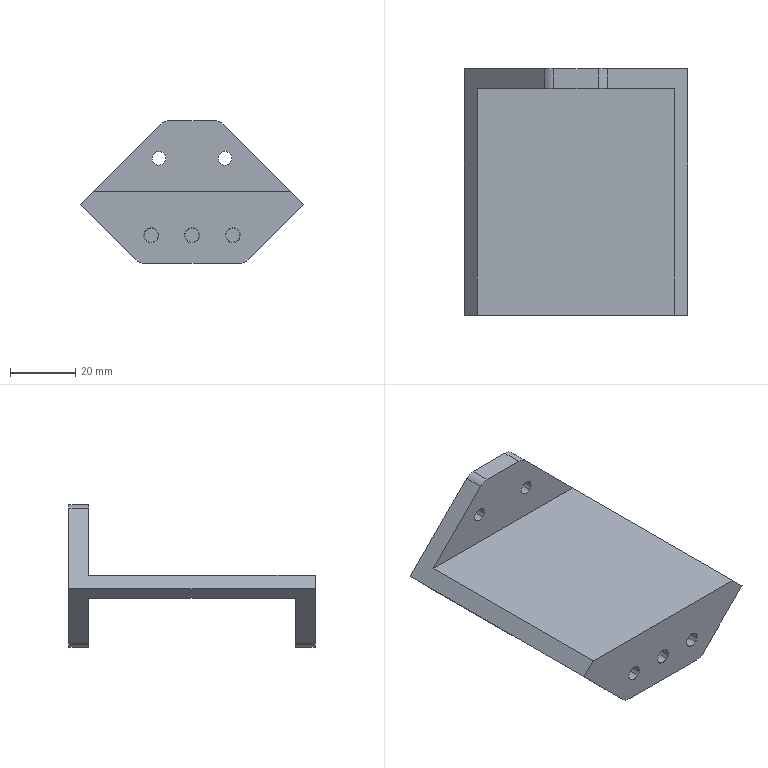NC program | NX | posted with a generic post | part box 68.307 x 75.3 x 43.668 mm
Lines 1 to 80 of 6865:
N10 G17 G21 G94 G90
(FLOOR_WALL_COPY_COPY , TOOL : D80)
N12 T19 M6
N14 G54
N16 G17 G0 G90 X-79.153 Y37.647 B0. C0. S6500 M3
N18 G43 Z30. H19
N20 Z9.
N22 G94 G1 Z6. F1500.
N24 X-74.153
N26 X74.153
N28 Y-5.65
N30 X-74.153
N32 X-79.153
N34 Z9.
N36 G0 Z30.
N38 Y37.647
N40 Z8.
N42 G1 Z5.
N44 X-74.153
N46 X74.153
N48 Y-5.65
N50 X-74.153
N52 X-79.153
N54 Z8.
N56 G0 Z30.
N58 Y37.647
N60 Z7.
N62 G1 Z4.
N64 X-74.153
N66 X74.153
N68 Y-5.65
N70 X-74.153
N72 X-79.153
N74 Z7.
N76 G0 Z30.
N78 Y37.647
N80 Z6.
N82 G1 Z3.
N84 X-74.153
N86 X74.153
N88 Y-5.65
N90 X-74.153
N92 X-79.153
N94 Z6.
N96 G0 Z30.
N98 Y37.647
N100 Z5.
N102 G1 Z2.
N104 X-74.153
N106 X74.153
N108 Y-5.65
N110 X-74.153
N112 X-79.153
N114 Z5.
N116 G0 Z30.
N118 Y37.647
N120 Z4.
N122 G1 Z1.
N124 X-74.153
N126 X74.153
N128 Y-5.65
N130 X-74.153
N132 X-79.153
N134 Z4.
N136 G0 Z30.
N138 Y37.647
N140 Z3.
N142 G1 Z0.
N144 X-74.153
N146 X74.153
N148 Y-5.65
N150 X-74.153
N152 X-79.153
N154 Z3.
N156 G0 Z30.
N158 M5